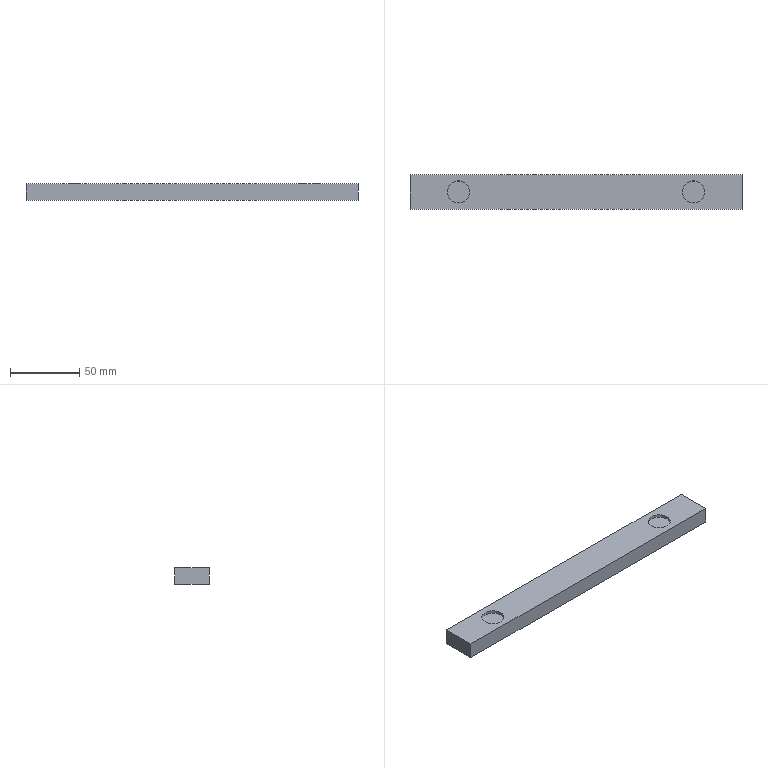Part | SolidWorks | features Extrusion 1, ICE 1 | 1 solid | 12 faces | box 240 x 25 x 12 mm | volume 71196 mm3 | plane 8 | cylinder 4 | commonest cylinder face diameters 16 x4
STEP:
#1=CARTESIAN_POINT('',(77.,0.,10.));
#2=VERTEX_POINT('',#1);
#3=CARTESIAN_POINT('',(93.,0.,10.));
#4=VERTEX_POINT('',#3);
#5=CARTESIAN_POINT('',(85.,0.,10.));
#6=DIRECTION('',(0.,0.,1.));
#7=DIRECTION('',(1.,0.,0.));
#8=AXIS2_PLACEMENT_3D('',#5,#6,#7);
#9=CIRCLE('',#8,8.);
#10=EDGE_CURVE('',#2,#4,#9,.T.);
#11=ORIENTED_EDGE('',*,*,#10,.F.);
#12=CARTESIAN_POINT('',(77.,0.,12.));
#13=VERTEX_POINT('',#12);
#14=CARTESIAN_POINT('',(77.,0.,10.));
#15=DIRECTION('',(0.,0.,1.));
#16=VECTOR('',#15,1000.);
#17=LINE('',#14,#16);
#18=EDGE_CURVE('',#2,#13,#17,.T.);
#19=ORIENTED_EDGE('',*,*,#18,.T.);
#20=CARTESIAN_POINT('',(93.,0.,12.));
#21=VERTEX_POINT('',#20);
#22=CARTESIAN_POINT('',(85.,0.,12.));
#23=DIRECTION('',(0.,0.,1.));
#24=DIRECTION('',(1.,0.,0.));
#25=AXIS2_PLACEMENT_3D('',#22,#23,#24);
#26=CIRCLE('',#25,8.);
#27=EDGE_CURVE('',#13,#21,#26,.T.);
#28=ORIENTED_EDGE('',*,*,#27,.T.);
#29=CARTESIAN_POINT('',(93.,0.,10.));
#30=DIRECTION('',(0.,0.,1.));
#31=VECTOR('',#30,1000.);
#32=LINE('',#29,#31);
#33=EDGE_CURVE('',#4,#21,#32,.T.);
#34=ORIENTED_EDGE('',*,*,#33,.F.);
#35=EDGE_LOOP('',(#11,#19,#28,#34));
#36=FACE_OUTER_BOUND('',#35,.T.);
#37=CARTESIAN_POINT('',(85.,0.,10.));
#38=DIRECTION('',(0.,0.,1.));
#39=DIRECTION('',(1.,0.,0.));
#40=AXIS2_PLACEMENT_3D('',#37,#38,#39);
#41=CYLINDRICAL_SURFACE('',#40,8.);
#42=ADVANCED_FACE('',(#36),#41,.F.);
#43=CARTESIAN_POINT('',(-93.,0.,10.));
#44=VERTEX_POINT('',#43);
#45=CARTESIAN_POINT('',(-77.,0.,10.));
#46=VERTEX_POINT('',#45);
#47=CARTESIAN_POINT('',(-85.,0.,10.));
#48=DIRECTION('',(0.,0.,1.));
#49=DIRECTION('',(1.,0.,0.));
#50=AXIS2_PLACEMENT_3D('',#47,#48,#49);
#51=CIRCLE('',#50,8.);
#52=EDGE_CURVE('',#44,#46,#51,.T.);
#53=ORIENTED_EDGE('',*,*,#52,.F.);
#54=CARTESIAN_POINT('',(-93.,0.,12.));
#55=VERTEX_POINT('',#54);
#56=CARTESIAN_POINT('',(-93.,0.,10.));
#57=DIRECTION('',(0.,0.,1.));
#58=VECTOR('',#57,1000.);
#59=LINE('',#56,#58);
#60=EDGE_CURVE('',#44,#55,#59,.T.);
#61=ORIENTED_EDGE('',*,*,#60,.T.);
#62=CARTESIAN_POINT('',(-77.,0.,12.));
#63=VERTEX_POINT('',#62);
#64=CARTESIAN_POINT('',(-85.,0.,12.));
#65=DIRECTION('',(0.,0.,1.));
#66=DIRECTION('',(1.,0.,0.));
#67=AXIS2_PLACEMENT_3D('',#64,#65,#66);
#68=CIRCLE('',#67,8.);
#69=EDGE_CURVE('',#55,#63,#68,.T.);
#70=ORIENTED_EDGE('',*,*,#69,.T.);
#71=CARTESIAN_POINT('',(-77.,0.,10.));
#72=DIRECTION('',(0.,0.,1.));
#73=VECTOR('',#72,1000.);
#74=LINE('',#71,#73);
#75=EDGE_CURVE('',#46,#63,#74,.T.);
#76=ORIENTED_EDGE('',*,*,#75,.F.);
#77=EDGE_LOOP('',(#53,#61,#70,#76));
#78=FACE_OUTER_BOUND('',#77,.T.);
#79=CARTESIAN_POINT('',(-85.,0.,10.));
#80=DIRECTION('',(0.,0.,1.));
#81=DIRECTION('',(1.,0.,0.));
#82=AXIS2_PLACEMENT_3D('',#79,#80,#81);
#83=CYLINDRICAL_SURFACE('',#82,8.);
#84=ADVANCED_FACE('',(#78),#83,.F.);
#85=CARTESIAN_POINT('',(120.,-12.5,0.));
#86=VERTEX_POINT('',#85);
#87=CARTESIAN_POINT('',(120.,12.5,0.));
#88=VERTEX_POINT('',#87);
#89=CARTESIAN_POINT('',(120.,-12.5,0.));
#90=DIRECTION('',(0.,1.,0.));
#91=VECTOR('',#90,1000.);
#92=LINE('',#89,#91);
#93=EDGE_CURVE('',#86,#88,#92,.T.);
#94=ORIENTED_EDGE('',*,*,#93,.T.);
#95=CARTESIAN_POINT('',(120.,12.5,12.));
#96=VERTEX_POINT('',#95);
#97=CARTESIAN_POINT('',(120.,12.5,12.));
#98=DIRECTION('',(0.,0.,-1.));
#99=VECTOR('',#98,1000.);
#100=LINE('',#97,#99);
#101=EDGE_CURVE('',#96,#88,#100,.T.);
#102=ORIENTED_EDGE('',*,*,#101,.F.);
#103=CARTESIAN_POINT('',(120.,-12.5,12.));
#104=VERTEX_POINT('',#103);
#105=CARTESIAN_POINT('',(120.,-12.5,12.));
#106=DIRECTION('',(0.,1.,0.));
#107=VECTOR('',#106,1000.);
#108=LINE('',#105,#107);
#109=EDGE_CURVE('',#104,#96,#108,.T.);
#110=ORIENTED_EDGE('',*,*,#109,.F.);
#111=CARTESIAN_POINT('',(120.,-12.5,12.));
#112=DIRECTION('',(0.,0.,-1.));
#113=VECTOR('',#112,1000.);
#114=LINE('',#111,#113);
#115=EDGE_CURVE('',#104,#86,#114,.T.);
#116=ORIENTED_EDGE('',*,*,#115,.T.);
#117=EDGE_LOOP('',(#94,#102,#110,#116));
#118=FACE_OUTER_BOUND('',#117,.T.);
#119=CARTESIAN_POINT('',(120.,-12.5,12.));
#120=DIRECTION('',(-1.,0.,0.));
#121=DIRECTION('',(0.,0.,1.));
#122=AXIS2_PLACEMENT_3D('',#119,#120,#121);
#123=PLANE('',#122);
#124=ADVANCED_FACE('',(#118),#123,.F.);
#125=CARTESIAN_POINT('',(-120.,12.5,0.));
#126=VERTEX_POINT('',#125);
#127=CARTESIAN_POINT('',(-120.,12.5,0.));
#128=DIRECTION('',(-1.,0.,0.));
#129=VECTOR('',#128,1000.);
#130=LINE('',#127,#129);
#131=EDGE_CURVE('',#88,#126,#130,.T.);
#132=ORIENTED_EDGE('',*,*,#131,.T.);
#133=CARTESIAN_POINT('',(-120.,12.5,12.));
#134=VERTEX_POINT('',#133);
#135=CARTESIAN_POINT('',(-120.,12.5,12.));
#136=DIRECTION('',(0.,0.,-1.));
#137=VECTOR('',#136,1000.);
#138=LINE('',#135,#137);
#139=EDGE_CURVE('',#134,#126,#138,.T.);
#140=ORIENTED_EDGE('',*,*,#139,.F.);
#141=CARTESIAN_POINT('',(-120.,12.5,12.));
#142=DIRECTION('',(-1.,0.,0.));
#143=VECTOR('',#142,1000.);
#144=LINE('',#141,#143);
#145=EDGE_CURVE('',#96,#134,#144,.T.);
#146=ORIENTED_EDGE('',*,*,#145,.F.);
#147=ORIENTED_EDGE('',*,*,#101,.T.);
#148=EDGE_LOOP('',(#132,#140,#146,#147));
#149=FACE_OUTER_BOUND('',#148,.T.);
#150=CARTESIAN_POINT('',(-120.,12.5,12.));
#151=DIRECTION('',(0.,-1.,0.));
#152=DIRECTION('',(0.,0.,-1.));
#153=AXIS2_PLACEMENT_3D('',#150,#151,#152);
#154=PLANE('',#153);
#155=ADVANCED_FACE('',(#149),#154,.F.);
#156=CARTESIAN_POINT('',(-120.,-12.5,0.));
#157=VERTEX_POINT('',#156);
#158=CARTESIAN_POINT('',(-120.,-12.5,0.));
#159=DIRECTION('',(0.,-1.,0.));
#160=VECTOR('',#159,1000.);
#161=LINE('',#158,#160);
#162=EDGE_CURVE('',#126,#157,#161,.T.);
#163=ORIENTED_EDGE('',*,*,#162,.T.);
#164=CARTESIAN_POINT('',(-120.,-12.5,12.));
#165=VERTEX_POINT('',#164);
#166=CARTESIAN_POINT('',(-120.,-12.5,12.));
#167=DIRECTION('',(0.,0.,-1.));
#168=VECTOR('',#167,1000.);
#169=LINE('',#166,#168);
#170=EDGE_CURVE('',#165,#157,#169,.T.);
#171=ORIENTED_EDGE('',*,*,#170,.F.);
#172=CARTESIAN_POINT('',(-120.,-12.5,12.));
#173=DIRECTION('',(0.,-1.,0.));
#174=VECTOR('',#173,1000.);
#175=LINE('',#172,#174);
#176=EDGE_CURVE('',#134,#165,#175,.T.);
#177=ORIENTED_EDGE('',*,*,#176,.F.);
#178=ORIENTED_EDGE('',*,*,#139,.T.);
#179=EDGE_LOOP('',(#163,#171,#177,#178));
#180=FACE_OUTER_BOUND('',#179,.T.);
#181=CARTESIAN_POINT('',(-120.,-12.5,12.));
#182=DIRECTION('',(1.,0.,0.));
#183=DIRECTION('',(0.,0.,-1.));
#184=AXIS2_PLACEMENT_3D('',#181,#182,#183);
#185=PLANE('',#184);
#186=ADVANCED_FACE('',(#180),#185,.F.);
#187=CARTESIAN_POINT('',(-120.,-12.5,0.));
#188=DIRECTION('',(1.,0.,0.));
#189=VECTOR('',#188,1000.);
#190=LINE('',#187,#189);
#191=EDGE_CURVE('',#157,#86,#190,.T.);
#192=ORIENTED_EDGE('',*,*,#191,.T.);
#193=ORIENTED_EDGE('',*,*,#115,.F.);
#194=CARTESIAN_POINT('',(-120.,-12.5,12.));
#195=DIRECTION('',(1.,0.,0.));
#196=VECTOR('',#195,1000.);
#197=LINE('',#194,#196);
#198=EDGE_CURVE('',#165,#104,#197,.T.);
#199=ORIENTED_EDGE('',*,*,#198,.F.);
#200=ORIENTED_EDGE('',*,*,#170,.T.);
#201=EDGE_LOOP('',(#192,#193,#199,#200));
#202=FACE_OUTER_BOUND('',#201,.T.);
#203=CARTESIAN_POINT('',(-120.,-12.5,12.));
#204=DIRECTION('',(0.,1.,0.));
#205=DIRECTION('',(0.,0.,1.));
#206=AXIS2_PLACEMENT_3D('',#203,#204,#205);
#207=PLANE('',#206);
#208=ADVANCED_FACE('',(#202),#207,.F.);
#209=CARTESIAN_POINT('',(85.,0.,12.));
#210=DIRECTION('',(0.,0.,1.));
#211=DIRECTION('',(1.,0.,0.));
#212=AXIS2_PLACEMENT_3D('',#209,#210,#211);
#213=CIRCLE('',#212,8.);
#214=EDGE_CURVE('',#21,#13,#213,.T.);
#215=ORIENTED_EDGE('',*,*,#214,.F.);
#216=ORIENTED_EDGE('',*,*,#27,.F.);
#217=EDGE_LOOP('',(#215,#216));
#218=FACE_BOUND('',#217,.T.);
#219=CARTESIAN_POINT('',(-85.,0.,12.));
#220=DIRECTION('',(0.,0.,1.));
#221=DIRECTION('',(1.,0.,0.));
#222=AXIS2_PLACEMENT_3D('',#219,#220,#221);
#223=CIRCLE('',#222,8.);
#224=EDGE_CURVE('',#63,#55,#223,.T.);
#225=ORIENTED_EDGE('',*,*,#224,.F.);
#226=ORIENTED_EDGE('',*,*,#69,.F.);
#227=EDGE_LOOP('',(#225,#226));
#228=FACE_BOUND('',#227,.T.);
#229=ORIENTED_EDGE('',*,*,#109,.T.);
#230=ORIENTED_EDGE('',*,*,#145,.T.);
#231=ORIENTED_EDGE('',*,*,#176,.T.);
#232=ORIENTED_EDGE('',*,*,#198,.T.);
#233=EDGE_LOOP('',(#229,#230,#231,#232));
#234=FACE_OUTER_BOUND('',#233,.T.);
#235=CARTESIAN_POINT('',(0.,0.,12.));
#236=DIRECTION('',(0.,0.,-1.));
#237=DIRECTION('',(-1.,0.,0.));
#238=AXIS2_PLACEMENT_3D('',#235,#236,#237);
#239=PLANE('',#238);
#240=ADVANCED_FACE('',(#218,#228,#234),#239,.F.);
#241=ORIENTED_EDGE('',*,*,#93,.F.);
#242=ORIENTED_EDGE('',*,*,#191,.F.);
#243=ORIENTED_EDGE('',*,*,#162,.F.);
#244=ORIENTED_EDGE('',*,*,#131,.F.);
#245=EDGE_LOOP('',(#241,#242,#243,#244));
#246=FACE_OUTER_BOUND('',#245,.T.);
#247=CARTESIAN_POINT('',(0.,0.,0.));
#248=DIRECTION('',(0.,0.,-1.));
#249=DIRECTION('',(-1.,0.,0.));
#250=AXIS2_PLACEMENT_3D('',#247,#248,#249);
#251=PLANE('',#250);
#252=ADVANCED_FACE('',(#246),#251,.T.);
#253=ORIENTED_EDGE('',*,*,#60,.F.);
#254=CARTESIAN_POINT('',(-85.,0.,10.));
#255=DIRECTION('',(0.,0.,1.));
#256=DIRECTION('',(1.,0.,0.));
#257=AXIS2_PLACEMENT_3D('',#254,#255,#256);
#258=CIRCLE('',#257,8.);
#259=EDGE_CURVE('',#46,#44,#258,.T.);
#260=ORIENTED_EDGE('',*,*,#259,.F.);
#261=ORIENTED_EDGE('',*,*,#75,.T.);
#262=ORIENTED_EDGE('',*,*,#224,.T.);
#263=EDGE_LOOP('',(#253,#260,#261,#262));
#264=FACE_OUTER_BOUND('',#263,.T.);
#265=CARTESIAN_POINT('',(-85.,0.,10.));
#266=DIRECTION('',(0.,0.,1.));
#267=DIRECTION('',(1.,0.,0.));
#268=AXIS2_PLACEMENT_3D('',#265,#266,#267);
#269=CYLINDRICAL_SURFACE('',#268,8.);
#270=ADVANCED_FACE('',(#264),#269,.F.);
#271=ORIENTED_EDGE('',*,*,#259,.T.);
#272=ORIENTED_EDGE('',*,*,#52,.T.);
#273=EDGE_LOOP('',(#271,#272));
#274=FACE_OUTER_BOUND('',#273,.T.);
#275=CARTESIAN_POINT('',(-85.,0.,10.));
#276=DIRECTION('',(0.,0.,1.));
#277=DIRECTION('',(1.,0.,0.));
#278=AXIS2_PLACEMENT_3D('',#275,#276,#277);
#279=PLANE('',#278);
#280=ADVANCED_FACE('',(#274),#279,.T.);
#281=ORIENTED_EDGE('',*,*,#18,.F.);
#282=CARTESIAN_POINT('',(85.,0.,10.));
#283=DIRECTION('',(0.,0.,1.));
#284=DIRECTION('',(1.,0.,0.));
#285=AXIS2_PLACEMENT_3D('',#282,#283,#284);
#286=CIRCLE('',#285,8.);
#287=EDGE_CURVE('',#4,#2,#286,.T.);
#288=ORIENTED_EDGE('',*,*,#287,.F.);
#289=ORIENTED_EDGE('',*,*,#33,.T.);
#290=ORIENTED_EDGE('',*,*,#214,.T.);
#291=EDGE_LOOP('',(#281,#288,#289,#290));
#292=FACE_OUTER_BOUND('',#291,.T.);
#293=CARTESIAN_POINT('',(85.,0.,10.));
#294=DIRECTION('',(0.,0.,1.));
#295=DIRECTION('',(1.,0.,0.));
#296=AXIS2_PLACEMENT_3D('',#293,#294,#295);
#297=CYLINDRICAL_SURFACE('',#296,8.);
#298=ADVANCED_FACE('',(#292),#297,.F.);
#299=ORIENTED_EDGE('',*,*,#287,.T.);
#300=ORIENTED_EDGE('',*,*,#10,.T.);
#301=EDGE_LOOP('',(#299,#300));
#302=FACE_OUTER_BOUND('',#301,.T.);
#303=CARTESIAN_POINT('',(85.,0.,10.));
#304=DIRECTION('',(0.,0.,1.));
#305=DIRECTION('',(1.,0.,0.));
#306=AXIS2_PLACEMENT_3D('',#303,#304,#305);
#307=PLANE('',#306);
#308=ADVANCED_FACE('',(#302),#307,.T.);
#309=CLOSED_SHELL('',(#42,#84,#124,#155,#186,#208,#240,#252,#270,#280,#298,#308));
#310=MANIFOLD_SOLID_BREP('',#309);
#311=CARTESIAN_POINT('',(0.,0.,0.));
#312=DIRECTION('',(0.,0.,1.));
#313=DIRECTION('',(1.,0.,0.));
#314=AXIS2_PLACEMENT_3D('',#311,#312,#313);
#315=(LENGTH_UNIT()NAMED_UNIT(*)SI_UNIT(.MILLI.,.METRE.));
#316=UNCERTAINTY_MEASURE_WITH_UNIT(LENGTH_MEASURE(0.00001),#315,'','');
#317=(NAMED_UNIT(*)PLANE_ANGLE_UNIT()SI_UNIT($,.RADIAN.));
#318=(NAMED_UNIT(*)SI_UNIT($,.STERADIAN.)SOLID_ANGLE_UNIT());
#319=(GEOMETRIC_REPRESENTATION_CONTEXT(3)GLOBAL_UNCERTAINTY_ASSIGNED_CONTEXT((#316))GLOBAL_UNIT_ASSIGNED_CONTEXT((#315,#317,#318))REPRESENTATION_CONTEXT('',''));
#320=ADVANCED_BREP_SHAPE_REPRESENTATION('',(#310,#314),#319);